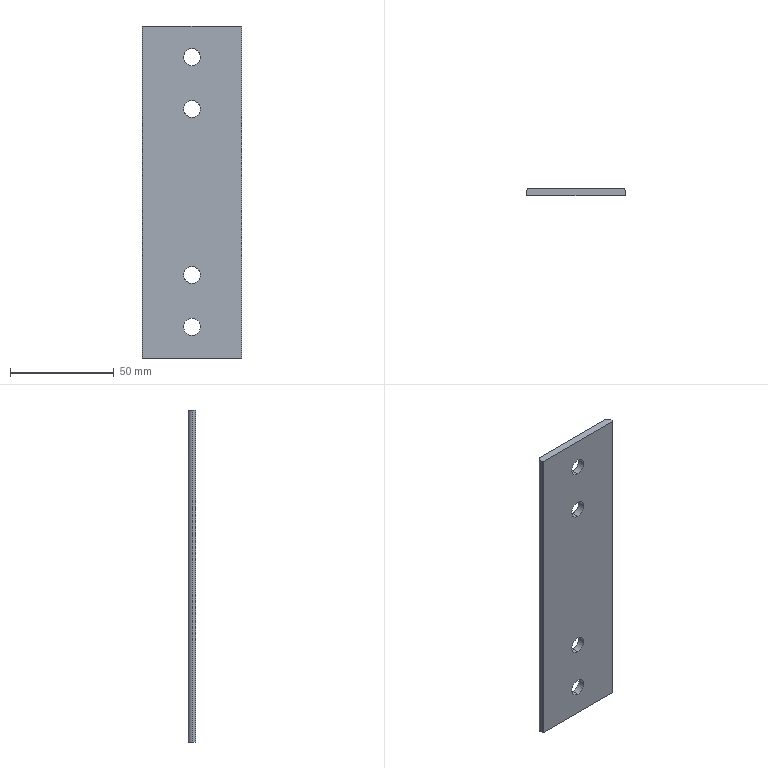Part | STEP file | 31E-01027QY13 | 1 solid | 18 faces | box 48 x 3.5 x 160 mm | volume 25860 mm3 | cylinder 12 | plane 6 | commonest cylinder face diameters 8.2 x8 0.6 x2 4 x2
STEP:
#1=CARTESIAN_POINT('',(0.,-1.75,10.9));
#2=VERTEX_POINT('',#1);
#3=CARTESIAN_POINT('',(0.,-1.75,19.1));
#4=VERTEX_POINT('',#3);
#5=CARTESIAN_POINT('',(0.,-1.75,15.));
#6=DIRECTION('',(0.,1.,0.));
#7=AXIS2_PLACEMENT_3D('',#5,#6,$);
#8=CIRCLE('',#7,4.1);
#9=EDGE_CURVE('',#2,#4,#8,.T.);
#10=ORIENTED_EDGE('',*,*,#9,.F.);
#11=CARTESIAN_POINT('',(0.,1.75,10.9));
#12=VERTEX_POINT('',#11);
#13=CARTESIAN_POINT('',(0.,-1.75,10.9));
#14=DIRECTION('',(0.,1.,0.));
#15=VECTOR('',#14,1.);
#16=LINE('',#13,#15);
#17=EDGE_CURVE('',#2,#12,#16,.T.);
#18=ORIENTED_EDGE('',*,*,#17,.T.);
#19=CARTESIAN_POINT('',(0.,1.75,19.1));
#20=VERTEX_POINT('',#19);
#21=CARTESIAN_POINT('',(0.,1.75,15.));
#22=DIRECTION('',(0.,1.,0.));
#23=AXIS2_PLACEMENT_3D('',#21,#22,$);
#24=CIRCLE('',#23,4.1);
#25=EDGE_CURVE('',#12,#20,#24,.T.);
#26=ORIENTED_EDGE('',*,*,#25,.T.);
#27=CARTESIAN_POINT('',(0.,-1.75,19.1));
#28=DIRECTION('',(0.,1.,0.));
#29=VECTOR('',#28,1.);
#30=LINE('',#27,#29);
#31=EDGE_CURVE('',#4,#20,#30,.T.);
#32=ORIENTED_EDGE('',*,*,#31,.F.);
#33=EDGE_LOOP('',(#10,#18,#26,#32));
#34=FACE_OUTER_BOUND('',#33,.T.);
#35=CARTESIAN_POINT('',(0.,-1.75,15.));
#36=DIRECTION('',(0.,1.,0.));
#37=DIRECTION('',(0.,0.,-1.));
#38=AXIS2_PLACEMENT_3D('',#35,#36,#37);
#39=CYLINDRICAL_SURFACE('',#38,4.1);
#40=ADVANCED_FACE('',(#34),#39,.F.);
#41=CARTESIAN_POINT('',(-23.7,-1.75,160.));
#42=VERTEX_POINT('',#41);
#43=CARTESIAN_POINT('',(23.7,-1.75,160.));
#44=VERTEX_POINT('',#43);
#45=CARTESIAN_POINT('',(0.,-1.75,160.));
#46=DIRECTION('',(1.,0.,0.));
#47=VECTOR('',#46,1.);
#48=LINE('',#45,#47);
#49=EDGE_CURVE('',#42,#44,#48,.T.);
#50=ORIENTED_EDGE('',*,*,#49,.F.);
#51=CARTESIAN_POINT('',(-23.7,-1.75,0.));
#52=VERTEX_POINT('',#51);
#53=CARTESIAN_POINT('',(-23.7,-1.75,80.));
#54=DIRECTION('',(0.,0.,-1.));
#55=VECTOR('',#54,1.);
#56=LINE('',#53,#55);
#57=EDGE_CURVE('',#42,#52,#56,.T.);
#58=ORIENTED_EDGE('',*,*,#57,.T.);
#59=CARTESIAN_POINT('',(23.7,-1.75,0.));
#60=VERTEX_POINT('',#59);
#61=CARTESIAN_POINT('',(0.,-1.75,0.));
#62=DIRECTION('',(1.,0.,0.));
#63=VECTOR('',#62,1.);
#64=LINE('',#61,#63);
#65=EDGE_CURVE('',#52,#60,#64,.T.);
#66=ORIENTED_EDGE('',*,*,#65,.T.);
#67=CARTESIAN_POINT('',(23.7,-1.75,80.));
#68=DIRECTION('',(0.,0.,1.));
#69=VECTOR('',#68,1.);
#70=LINE('',#67,#69);
#71=EDGE_CURVE('',#60,#44,#70,.T.);
#72=ORIENTED_EDGE('',*,*,#71,.T.);
#73=EDGE_LOOP('',(#50,#58,#66,#72));
#74=FACE_OUTER_BOUND('',#73,.T.);
#75=CARTESIAN_POINT('',(0.,-1.75,15.));
#76=DIRECTION('',(0.,1.,0.));
#77=AXIS2_PLACEMENT_3D('',#75,#76,$);
#78=CIRCLE('',#77,4.1);
#79=EDGE_CURVE('',#4,#2,#78,.T.);
#80=ORIENTED_EDGE('',*,*,#79,.T.);
#81=ORIENTED_EDGE('',*,*,#9,.T.);
#82=EDGE_LOOP('',(#80,#81));
#83=FACE_BOUND('',#82,.T.);
#84=CARTESIAN_POINT('',(0.,-1.75,44.1));
#85=VERTEX_POINT('',#84);
#86=CARTESIAN_POINT('',(0.,-1.75,35.9));
#87=VERTEX_POINT('',#86);
#88=CARTESIAN_POINT('',(0.,-1.75,40.));
#89=DIRECTION('',(0.,1.,0.));
#90=AXIS2_PLACEMENT_3D('',#88,#89,$);
#91=CIRCLE('',#90,4.1);
#92=EDGE_CURVE('',#85,#87,#91,.T.);
#93=ORIENTED_EDGE('',*,*,#92,.T.);
#94=CARTESIAN_POINT('',(0.,-1.75,40.));
#95=DIRECTION('',(0.,1.,0.));
#96=AXIS2_PLACEMENT_3D('',#94,#95,$);
#97=CIRCLE('',#96,4.1);
#98=EDGE_CURVE('',#87,#85,#97,.T.);
#99=ORIENTED_EDGE('',*,*,#98,.T.);
#100=EDGE_LOOP('',(#93,#99));
#101=FACE_BOUND('',#100,.T.);
#102=CARTESIAN_POINT('',(0.,-1.75,149.1));
#103=VERTEX_POINT('',#102);
#104=CARTESIAN_POINT('',(0.,-1.75,140.9));
#105=VERTEX_POINT('',#104);
#106=CARTESIAN_POINT('',(0.,-1.75,145.));
#107=DIRECTION('',(0.,1.,0.));
#108=AXIS2_PLACEMENT_3D('',#106,#107,$);
#109=CIRCLE('',#108,4.1);
#110=EDGE_CURVE('',#103,#105,#109,.T.);
#111=ORIENTED_EDGE('',*,*,#110,.T.);
#112=CARTESIAN_POINT('',(0.,-1.75,145.));
#113=DIRECTION('',(0.,1.,0.));
#114=AXIS2_PLACEMENT_3D('',#112,#113,$);
#115=CIRCLE('',#114,4.1);
#116=EDGE_CURVE('',#105,#103,#115,.T.);
#117=ORIENTED_EDGE('',*,*,#116,.T.);
#118=EDGE_LOOP('',(#111,#117));
#119=FACE_BOUND('',#118,.T.);
#120=CARTESIAN_POINT('',(0.,-1.75,124.1));
#121=VERTEX_POINT('',#120);
#122=CARTESIAN_POINT('',(0.,-1.75,115.9));
#123=VERTEX_POINT('',#122);
#124=CARTESIAN_POINT('',(0.,-1.75,120.));
#125=DIRECTION('',(0.,1.,0.));
#126=AXIS2_PLACEMENT_3D('',#124,#125,$);
#127=CIRCLE('',#126,4.1);
#128=EDGE_CURVE('',#121,#123,#127,.T.);
#129=ORIENTED_EDGE('',*,*,#128,.T.);
#130=CARTESIAN_POINT('',(0.,-1.75,120.));
#131=DIRECTION('',(0.,1.,0.));
#132=AXIS2_PLACEMENT_3D('',#130,#131,$);
#133=CIRCLE('',#132,4.1);
#134=EDGE_CURVE('',#123,#121,#133,.T.);
#135=ORIENTED_EDGE('',*,*,#134,.T.);
#136=EDGE_LOOP('',(#129,#135));
#137=FACE_BOUND('',#136,.T.);
#138=CARTESIAN_POINT('',(-24.,-1.75,160.));
#139=DIRECTION('',(0.,1.,0.));
#140=DIRECTION('',(0.,0.,1.));
#141=AXIS2_PLACEMENT_3D('',#138,#139,#140);
#142=PLANE('',#141);
#143=ADVANCED_FACE('',(#74,#83,#101,#119,#137),#142,.F.);
#144=ORIENTED_EDGE('',*,*,#17,.F.);
#145=ORIENTED_EDGE('',*,*,#79,.F.);
#146=ORIENTED_EDGE('',*,*,#31,.T.);
#147=CARTESIAN_POINT('',(0.,1.75,15.));
#148=DIRECTION('',(0.,1.,0.));
#149=AXIS2_PLACEMENT_3D('',#147,#148,$);
#150=CIRCLE('',#149,4.1);
#151=EDGE_CURVE('',#20,#12,#150,.T.);
#152=ORIENTED_EDGE('',*,*,#151,.T.);
#153=EDGE_LOOP('',(#144,#145,#146,#152));
#154=FACE_OUTER_BOUND('',#153,.T.);
#155=CARTESIAN_POINT('',(0.,-1.75,15.));
#156=DIRECTION('',(0.,1.,0.));
#157=DIRECTION('',(0.,0.,1.));
#158=AXIS2_PLACEMENT_3D('',#155,#156,#157);
#159=CYLINDRICAL_SURFACE('',#158,4.1);
#160=ADVANCED_FACE('',(#154),#159,.F.);
#161=CARTESIAN_POINT('',(22.,1.75,0.));
#162=VERTEX_POINT('',#161);
#163=CARTESIAN_POINT('',(-22.,1.75,0.));
#164=VERTEX_POINT('',#163);
#165=CARTESIAN_POINT('',(0.,1.75,0.));
#166=DIRECTION('',(-1.,0.,0.));
#167=VECTOR('',#166,1.);
#168=LINE('',#165,#167);
#169=EDGE_CURVE('',#162,#164,#168,.T.);
#170=ORIENTED_EDGE('',*,*,#169,.T.);
#171=CARTESIAN_POINT('',(-22.,1.75,160.));
#172=VERTEX_POINT('',#171);
#173=CARTESIAN_POINT('',(-22.,1.75,80.));
#174=DIRECTION('',(0.,0.,1.));
#175=VECTOR('',#174,1.);
#176=LINE('',#173,#175);
#177=EDGE_CURVE('',#164,#172,#176,.T.);
#178=ORIENTED_EDGE('',*,*,#177,.T.);
#179=CARTESIAN_POINT('',(22.,1.75,160.));
#180=VERTEX_POINT('',#179);
#181=CARTESIAN_POINT('',(0.,1.75,160.));
#182=DIRECTION('',(-1.,0.,0.));
#183=VECTOR('',#182,1.);
#184=LINE('',#181,#183);
#185=EDGE_CURVE('',#180,#172,#184,.T.);
#186=ORIENTED_EDGE('',*,*,#185,.F.);
#187=CARTESIAN_POINT('',(22.,1.75,80.));
#188=DIRECTION('',(0.,0.,-1.));
#189=VECTOR('',#188,1.);
#190=LINE('',#187,#189);
#191=EDGE_CURVE('',#180,#162,#190,.T.);
#192=ORIENTED_EDGE('',*,*,#191,.T.);
#193=EDGE_LOOP('',(#170,#178,#186,#192));
#194=FACE_OUTER_BOUND('',#193,.T.);
#195=ORIENTED_EDGE('',*,*,#151,.F.);
#196=ORIENTED_EDGE('',*,*,#25,.F.);
#197=EDGE_LOOP('',(#195,#196));
#198=FACE_BOUND('',#197,.T.);
#199=CARTESIAN_POINT('',(0.,1.75,44.1));
#200=VERTEX_POINT('',#199);
#201=CARTESIAN_POINT('',(0.,1.75,35.9));
#202=VERTEX_POINT('',#201);
#203=CARTESIAN_POINT('',(0.,1.75,44.1));
#204=CARTESIAN_POINT('',(0.3968,1.75,44.1));
#205=CARTESIAN_POINT('',(0.7936,1.75,44.052));
#206=CARTESIAN_POINT('',(1.183,1.75,43.956));
#207=CARTESIAN_POINT('',(1.93,1.75,43.672));
#208=CARTESIAN_POINT('',(2.588,1.75,43.218));
#209=CARTESIAN_POINT('',(2.887,1.75,42.952));
#210=CARTESIAN_POINT('',(3.416,1.75,42.352));
#211=CARTESIAN_POINT('',(3.787,1.75,41.644));
#212=CARTESIAN_POINT('',(3.929,1.75,41.27));
#213=CARTESIAN_POINT('',(4.119,1.75,40.493));
#214=CARTESIAN_POINT('',(4.118,1.75,39.694));
#215=CARTESIAN_POINT('',(4.069,1.75,39.296));
#216=CARTESIAN_POINT('',(3.875,1.75,38.52));
#217=CARTESIAN_POINT('',(3.502,1.75,37.813));
#218=CARTESIAN_POINT('',(3.274,1.75,37.484));
#219=CARTESIAN_POINT('',(2.742,1.75,36.887));
#220=CARTESIAN_POINT('',(2.083,1.75,36.435));
#221=CARTESIAN_POINT('',(1.728,1.75,36.25));
#222=CARTESIAN_POINT('',(1.169,1.75,36.04));
#223=CARTESIAN_POINT('',(0.5857,1.75,35.935));
#224=CARTESIAN_POINT('',(0.3903,1.75,35.912));
#225=CARTESIAN_POINT('',(0.1952,1.75,35.9));
#226=CARTESIAN_POINT('',(0.,1.75,35.9));
#227=B_SPLINE_CURVE_WITH_KNOTS('',5,(#203,#204,#205,#206,#207,#208,#209,#210,#211,#212,#213,#214,#215,#216,#217,#218,#219,#220,#221,#222,#223,#224,#225,#226),.UNSPECIFIED.,.F.,.U.,(6,3,3,3,3,3,3,6),(0.,2.806,5.611,8.417,11.223,14.028,16.834,18.214),.UNSPECIFIED.);
#228=EDGE_CURVE('',#200,#202,#227,.T.);
#229=ORIENTED_EDGE('',*,*,#228,.F.);
#230=CARTESIAN_POINT('',(0.,1.75,35.9));
#231=CARTESIAN_POINT('',(-0.3968,1.75,35.9));
#232=CARTESIAN_POINT('',(-0.7936,1.75,35.948));
#233=CARTESIAN_POINT('',(-1.183,1.75,36.044));
#234=CARTESIAN_POINT('',(-1.93,1.75,36.328));
#235=CARTESIAN_POINT('',(-2.588,1.75,36.782));
#236=CARTESIAN_POINT('',(-2.887,1.75,37.048));
#237=CARTESIAN_POINT('',(-3.416,1.75,37.648));
#238=CARTESIAN_POINT('',(-3.787,1.75,38.356));
#239=CARTESIAN_POINT('',(-3.929,1.75,38.73));
#240=CARTESIAN_POINT('',(-4.119,1.75,39.507));
#241=CARTESIAN_POINT('',(-4.118,1.75,40.306));
#242=CARTESIAN_POINT('',(-4.069,1.75,40.704));
#243=CARTESIAN_POINT('',(-3.875,1.75,41.48));
#244=CARTESIAN_POINT('',(-3.502,1.75,42.187));
#245=CARTESIAN_POINT('',(-3.274,1.75,42.516));
#246=CARTESIAN_POINT('',(-2.742,1.75,43.113));
#247=CARTESIAN_POINT('',(-2.083,1.75,43.565));
#248=CARTESIAN_POINT('',(-1.728,1.75,43.75));
#249=CARTESIAN_POINT('',(-1.169,1.75,43.96));
#250=CARTESIAN_POINT('',(-0.5857,1.75,44.065));
#251=CARTESIAN_POINT('',(-0.3903,1.75,44.088));
#252=CARTESIAN_POINT('',(-0.1952,1.75,44.1));
#253=CARTESIAN_POINT('',(0.,1.75,44.1));
#254=B_SPLINE_CURVE_WITH_KNOTS('',5,(#230,#231,#232,#233,#234,#235,#236,#237,#238,#239,#240,#241,#242,#243,#244,#245,#246,#247,#248,#249,#250,#251,#252,#253),.UNSPECIFIED.,.F.,.U.,(6,3,3,3,3,3,3,6),(0.,2.806,5.611,8.417,11.223,14.028,16.834,18.214),.UNSPECIFIED.);
#255=EDGE_CURVE('',#202,#200,#254,.T.);
#256=ORIENTED_EDGE('',*,*,#255,.F.);
#257=EDGE_LOOP('',(#229,#256));
#258=FACE_BOUND('',#257,.T.);
#259=CARTESIAN_POINT('',(0.,1.75,149.1));
#260=VERTEX_POINT('',#259);
#261=CARTESIAN_POINT('',(0.,1.75,140.9));
#262=VERTEX_POINT('',#261);
#263=CARTESIAN_POINT('',(0.,1.75,149.1));
#264=CARTESIAN_POINT('',(0.3968,1.75,149.1));
#265=CARTESIAN_POINT('',(0.7936,1.75,149.052));
#266=CARTESIAN_POINT('',(1.183,1.75,148.956));
#267=CARTESIAN_POINT('',(1.93,1.75,148.672));
#268=CARTESIAN_POINT('',(2.588,1.75,148.218));
#269=CARTESIAN_POINT('',(2.887,1.75,147.952));
#270=CARTESIAN_POINT('',(3.416,1.75,147.352));
#271=CARTESIAN_POINT('',(3.787,1.75,146.644));
#272=CARTESIAN_POINT('',(3.929,1.75,146.27));
#273=CARTESIAN_POINT('',(4.119,1.75,145.493));
#274=CARTESIAN_POINT('',(4.118,1.75,144.694));
#275=CARTESIAN_POINT('',(4.069,1.75,144.296));
#276=CARTESIAN_POINT('',(3.875,1.75,143.52));
#277=CARTESIAN_POINT('',(3.502,1.75,142.813));
#278=CARTESIAN_POINT('',(3.274,1.75,142.484));
#279=CARTESIAN_POINT('',(2.742,1.75,141.887));
#280=CARTESIAN_POINT('',(2.083,1.75,141.435));
#281=CARTESIAN_POINT('',(1.728,1.75,141.25));
#282=CARTESIAN_POINT('',(1.169,1.75,141.04));
#283=CARTESIAN_POINT('',(0.5857,1.75,140.935));
#284=CARTESIAN_POINT('',(0.3903,1.75,140.912));
#285=CARTESIAN_POINT('',(0.1952,1.75,140.9));
#286=CARTESIAN_POINT('',(0.,1.75,140.9));
#287=B_SPLINE_CURVE_WITH_KNOTS('',5,(#263,#264,#265,#266,#267,#268,#269,#270,#271,#272,#273,#274,#275,#276,#277,#278,#279,#280,#281,#282,#283,#284,#285,#286),.UNSPECIFIED.,.F.,.U.,(6,3,3,3,3,3,3,6),(0.,2.806,5.611,8.417,11.223,14.028,16.834,18.214),.UNSPECIFIED.);
#288=EDGE_CURVE('',#260,#262,#287,.T.);
#289=ORIENTED_EDGE('',*,*,#288,.F.);
#290=CARTESIAN_POINT('',(0.,1.75,140.9));
#291=CARTESIAN_POINT('',(-0.3968,1.75,140.9));
#292=CARTESIAN_POINT('',(-0.7936,1.75,140.948));
#293=CARTESIAN_POINT('',(-1.183,1.75,141.044));
#294=CARTESIAN_POINT('',(-1.93,1.75,141.328));
#295=CARTESIAN_POINT('',(-2.588,1.75,141.782));
#296=CARTESIAN_POINT('',(-2.887,1.75,142.048));
#297=CARTESIAN_POINT('',(-3.416,1.75,142.648));
#298=CARTESIAN_POINT('',(-3.787,1.75,143.356));
#299=CARTESIAN_POINT('',(-3.929,1.75,143.73));
#300=CARTESIAN_POINT('',(-4.119,1.75,144.507));
#301=CARTESIAN_POINT('',(-4.118,1.75,145.306));
#302=CARTESIAN_POINT('',(-4.069,1.75,145.704));
#303=CARTESIAN_POINT('',(-3.875,1.75,146.48));
#304=CARTESIAN_POINT('',(-3.502,1.75,147.187));
#305=CARTESIAN_POINT('',(-3.274,1.75,147.516));
#306=CARTESIAN_POINT('',(-2.742,1.75,148.113));
#307=CARTESIAN_POINT('',(-2.083,1.75,148.565));
#308=CARTESIAN_POINT('',(-1.728,1.75,148.75));
#309=CARTESIAN_POINT('',(-1.169,1.75,148.96));
#310=CARTESIAN_POINT('',(-0.5857,1.75,149.065));
#311=CARTESIAN_POINT('',(-0.3903,1.75,149.088));
#312=CARTESIAN_POINT('',(-0.1952,1.75,149.1));
#313=CARTESIAN_POINT('',(0.,1.75,149.1));
#314=B_SPLINE_CURVE_WITH_KNOTS('',5,(#290,#291,#292,#293,#294,#295,#296,#297,#298,#299,#300,#301,#302,#303,#304,#305,#306,#307,#308,#309,#310,#311,#312,#313),.UNSPECIFIED.,.F.,.U.,(6,3,3,3,3,3,3,6),(0.,2.806,5.611,8.417,11.223,14.028,16.834,18.214),.UNSPECIFIED.);
#315=EDGE_CURVE('',#262,#260,#314,.T.);
#316=ORIENTED_EDGE('',*,*,#315,.F.);
#317=EDGE_LOOP('',(#289,#316));
#318=FACE_BOUND('',#317,.T.);
#319=CARTESIAN_POINT('',(0.,1.75,124.1));
#320=VERTEX_POINT('',#319);
#321=CARTESIAN_POINT('',(0.,1.75,115.9));
#322=VERTEX_POINT('',#321);
#323=CARTESIAN_POINT('',(0.,1.75,124.1));
#324=CARTESIAN_POINT('',(0.3968,1.75,124.1));
#325=CARTESIAN_POINT('',(0.7936,1.75,124.052));
#326=CARTESIAN_POINT('',(1.183,1.75,123.956));
#327=CARTESIAN_POINT('',(1.93,1.75,123.672));
#328=CARTESIAN_POINT('',(2.588,1.75,123.218));
#329=CARTESIAN_POINT('',(2.887,1.75,122.952));
#330=CARTESIAN_POINT('',(3.416,1.75,122.352));
#331=CARTESIAN_POINT('',(3.787,1.75,121.644));
#332=CARTESIAN_POINT('',(3.929,1.75,121.27));
#333=CARTESIAN_POINT('',(4.119,1.75,120.493));
#334=CARTESIAN_POINT('',(4.118,1.75,119.694));
#335=CARTESIAN_POINT('',(4.069,1.75,119.296));
#336=CARTESIAN_POINT('',(3.875,1.75,118.52));
#337=CARTESIAN_POINT('',(3.502,1.75,117.813));
#338=CARTESIAN_POINT('',(3.274,1.75,117.484));
#339=CARTESIAN_POINT('',(2.742,1.75,116.887));
#340=CARTESIAN_POINT('',(2.083,1.75,116.435));
#341=CARTESIAN_POINT('',(1.728,1.75,116.25));
#342=CARTESIAN_POINT('',(1.169,1.75,116.04));
#343=CARTESIAN_POINT('',(0.5857,1.75,115.935));
#344=CARTESIAN_POINT('',(0.3903,1.75,115.912));
#345=CARTESIAN_POINT('',(0.1952,1.75,115.9));
#346=CARTESIAN_POINT('',(0.,1.75,115.9));
#347=B_SPLINE_CURVE_WITH_KNOTS('',5,(#323,#324,#325,#326,#327,#328,#329,#330,#331,#332,#333,#334,#335,#336,#337,#338,#339,#340,#341,#342,#343,#344,#345,#346),.UNSPECIFIED.,.F.,.U.,(6,3,3,3,3,3,3,6),(0.,2.806,5.611,8.417,11.223,14.028,16.834,18.214),.UNSPECIFIED.);
#348=EDGE_CURVE('',#320,#322,#347,.T.);
#349=ORIENTED_EDGE('',*,*,#348,.F.);
#350=CARTESIAN_POINT('',(0.,1.75,115.9));
#351=CARTESIAN_POINT('',(-0.3968,1.75,115.9));
#352=CARTESIAN_POINT('',(-0.7936,1.75,115.948));
#353=CARTESIAN_POINT('',(-1.183,1.75,116.044));
#354=CARTESIAN_POINT('',(-1.93,1.75,116.328));
#355=CARTESIAN_POINT('',(-2.588,1.75,116.782));
#356=CARTESIAN_POINT('',(-2.887,1.75,117.048));
#357=CARTESIAN_POINT('',(-3.416,1.75,117.648));
#358=CARTESIAN_POINT('',(-3.787,1.75,118.356));
#359=CARTESIAN_POINT('',(-3.929,1.75,118.73));
#360=CARTESIAN_POINT('',(-4.119,1.75,119.507));
#361=CARTESIAN_POINT('',(-4.118,1.75,120.306));
#362=CARTESIAN_POINT('',(-4.069,1.75,120.704));
#363=CARTESIAN_POINT('',(-3.875,1.75,121.48));
#364=CARTESIAN_POINT('',(-3.502,1.75,122.187));
#365=CARTESIAN_POINT('',(-3.274,1.75,122.516));
#366=CARTESIAN_POINT('',(-2.742,1.75,123.113));
#367=CARTESIAN_POINT('',(-2.083,1.75,123.565));
#368=CARTESIAN_POINT('',(-1.728,1.75,123.75));
#369=CARTESIAN_POINT('',(-1.169,1.75,123.96));
#370=CARTESIAN_POINT('',(-0.5857,1.75,124.065));
#371=CARTESIAN_POINT('',(-0.3903,1.75,124.088));
#372=CARTESIAN_POINT('',(-0.1952,1.75,124.1));
#373=CARTESIAN_POINT('',(0.,1.75,124.1));
#374=B_SPLINE_CURVE_WITH_KNOTS('',5,(#350,#351,#352,#353,#354,#355,#356,#357,#358,#359,#360,#361,#362,#363,#364,#365,#366,#367,#368,#369,#370,#371,#372,#373),.UNSPECIFIED.,.F.,.U.,(6,3,3,3,3,3,3,6),(0.,2.806,5.611,8.417,11.223,14.028,16.834,18.214),.UNSPECIFIED.);
#375=EDGE_CURVE('',#322,#320,#374,.T.);
#376=ORIENTED_EDGE('',*,*,#375,.F.);
#377=EDGE_LOOP('',(#349,#376));
#378=FACE_BOUND('',#377,.T.);
#379=CARTESIAN_POINT('',(-24.,1.75,160.));
#380=DIRECTION('',(0.,-1.,0.));
#381=DIRECTION('',(0.,0.,-1.));
#382=AXIS2_PLACEMENT_3D('',#379,#380,#381);
#383=PLANE('',#382);
#384=ADVANCED_FACE('',(#194,#198,#258,#318,#378),#383,.F.);
#385=CARTESIAN_POINT('',(-24.,-0.25,160.));
#386=VERTEX_POINT('',#385);
#387=CARTESIAN_POINT('',(-24.,-1.45,160.));
#388=VERTEX_POINT('',#387);
#389=CARTESIAN_POINT('',(-24.,-0.85,160.));
#390=DIRECTION('',(0.,-1.,0.));
#391=VECTOR('',#390,1.);
#392=LINE('',#389,#391);
#393=EDGE_CURVE('',#386,#388,#392,.T.);
#394=ORIENTED_EDGE('',*,*,#393,.T.);
#395=CARTESIAN_POINT('',(-23.7,-1.45,160.));
#396=DIRECTION('',(0.,0.,1.));
#397=AXIS2_PLACEMENT_3D('',#395,#396,$);
#398=CIRCLE('',#397,0.3);
#399=EDGE_CURVE('',#388,#42,#398,.T.);
#400=ORIENTED_EDGE('',*,*,#399,.T.);
#401=ORIENTED_EDGE('',*,*,#49,.T.);
#402=CARTESIAN_POINT('',(24.,-1.45,160.));
#403=VERTEX_POINT('',#402);
#404=CARTESIAN_POINT('',(23.7,-1.45,160.));
#405=DIRECTION('',(0.,0.,1.));
#406=AXIS2_PLACEMENT_3D('',#404,#405,$);
#407=CIRCLE('',#406,0.3);
#408=EDGE_CURVE('',#44,#403,#407,.T.);
#409=ORIENTED_EDGE('',*,*,#408,.T.);
#410=CARTESIAN_POINT('',(24.,-0.25,160.));
#411=VERTEX_POINT('',#410);
#412=CARTESIAN_POINT('',(24.,-0.85,160.));
#413=DIRECTION('',(0.,1.,0.));
#414=VECTOR('',#413,1.);
#415=LINE('',#412,#414);
#416=EDGE_CURVE('',#403,#411,#415,.T.);
#417=ORIENTED_EDGE('',*,*,#416,.T.);
#418=CARTESIAN_POINT('',(22.,-0.25,160.));
#419=DIRECTION('',(0.,0.,1.));
#420=AXIS2_PLACEMENT_3D('',#418,#419,$);
#421=CIRCLE('',#420,2.);
#422=EDGE_CURVE('',#411,#180,#421,.T.);
#423=ORIENTED_EDGE('',*,*,#422,.T.);
#424=ORIENTED_EDGE('',*,*,#185,.T.);
#425=CARTESIAN_POINT('',(-22.,-0.25,160.));
#426=DIRECTION('',(0.,0.,1.));
#427=AXIS2_PLACEMENT_3D('',#425,#426,$);
#428=CIRCLE('',#427,2.);
#429=EDGE_CURVE('',#172,#386,#428,.T.);
#430=ORIENTED_EDGE('',*,*,#429,.T.);
#431=EDGE_LOOP('',(#394,#400,#401,#409,#417,#423,#424,#430));
#432=FACE_OUTER_BOUND('',#431,.T.);
#433=CARTESIAN_POINT('',(24.,-1.75,160.));
#434=DIRECTION('',(0.,0.,1.));
#435=DIRECTION('',(1.,0.,0.));
#436=AXIS2_PLACEMENT_3D('',#433,#434,#435);
#437=PLANE('',#436);
#438=ADVANCED_FACE('',(#432),#437,.T.);
#439=ORIENTED_EDGE('',*,*,#399,.F.);
#440=CARTESIAN_POINT('',(-24.,-1.45,0.));
#441=VERTEX_POINT('',#440);
#442=CARTESIAN_POINT('',(-24.,-1.45,160.));
#443=DIRECTION('',(0.,0.,-1.));
#444=VECTOR('',#443,1.);
#445=LINE('',#442,#444);
#446=EDGE_CURVE('',#441,#388,#445,.F.);
#447=ORIENTED_EDGE('',*,*,#446,.F.);
#448=CARTESIAN_POINT('',(-23.7,-1.45,0.));
#449=DIRECTION('',(0.,0.,-1.));
#450=AXIS2_PLACEMENT_3D('',#448,#449,$);
#451=CIRCLE('',#450,0.3);
#452=EDGE_CURVE('',#52,#441,#451,.T.);
#453=ORIENTED_EDGE('',*,*,#452,.F.);
#454=ORIENTED_EDGE('',*,*,#57,.F.);
#455=EDGE_LOOP('',(#439,#447,#453,#454));
#456=FACE_OUTER_BOUND('',#455,.T.);
#457=CARTESIAN_POINT('',(-23.7,-1.45,160.));
#458=DIRECTION('',(0.,0.,-1.));
#459=DIRECTION('',(1.,0.,0.));
#460=AXIS2_PLACEMENT_3D('',#457,#458,#459);
#461=CYLINDRICAL_SURFACE('',#460,0.3);
#462=ADVANCED_FACE('',(#456),#461,.T.);
#463=ORIENTED_EDGE('',*,*,#65,.F.);
#464=ORIENTED_EDGE('',*,*,#452,.T.);
#465=CARTESIAN_POINT('',(-24.,-0.25,0.));
#466=VERTEX_POINT('',#465);
#467=CARTESIAN_POINT('',(-24.,-0.85,0.));
#468=DIRECTION('',(0.,-1.,0.));
#469=VECTOR('',#468,1.);
#470=LINE('',#467,#469);
#471=EDGE_CURVE('',#466,#441,#470,.T.);
#472=ORIENTED_EDGE('',*,*,#471,.F.);
#473=CARTESIAN_POINT('',(-24.,-0.25,0.));
#474=CARTESIAN_POINT('',(-24.,-0.04216,0.));
#475=CARTESIAN_POINT('',(-23.973,0.1657,0.));
#476=CARTESIAN_POINT('',(-23.919,0.3689,0.));
#477=CARTESIAN_POINT('',(-23.759,0.7565,0.));
#478=CARTESIAN_POINT('',(-23.506,1.091,0.));
#479=CARTESIAN_POINT('',(-23.358,1.24,0.));
#480=CARTESIAN_POINT('',(-23.027,1.497,0.));
#481=CARTESIAN_POINT('',(-22.642,1.661,0.));
#482=CARTESIAN_POINT('',(-22.439,1.718,0.));
#483=CARTESIAN_POINT('',(-22.227,1.748,0.));
#484=CARTESIAN_POINT('',(-22.014,1.75,0.));
#485=CARTESIAN_POINT('',(-22.01,1.75,0.));
#486=CARTESIAN_POINT('',(-22.005,1.75,0.));
#487=CARTESIAN_POINT('',(-22.,1.75,0.));
#488=B_SPLINE_CURVE_WITH_KNOTS('',5,(#473,#474,#475,#476,#477,#478,#479,#480,#481,#482,#483,#484,#485,#486,#487),.UNSPECIFIED.,.F.,.U.,(6,3,3,3,6),(0.,1.47,2.939,4.409,4.443),.UNSPECIFIED.);
#489=EDGE_CURVE('',#466,#164,#488,.T.);
#490=ORIENTED_EDGE('',*,*,#489,.T.);
#491=ORIENTED_EDGE('',*,*,#169,.F.);
#492=CARTESIAN_POINT('',(24.,-0.25,0.));
#493=VERTEX_POINT('',#492);
#494=CARTESIAN_POINT('',(22.,1.75,0.));
#495=CARTESIAN_POINT('',(22.208,1.75,0.));
#496=CARTESIAN_POINT('',(22.416,1.723,0.));
#497=CARTESIAN_POINT('',(22.619,1.669,0.));
#498=CARTESIAN_POINT('',(23.006,1.509,0.));
#499=CARTESIAN_POINT('',(23.341,1.256,0.));
#500=CARTESIAN_POINT('',(23.49,1.108,0.));
#501=CARTESIAN_POINT('',(23.747,0.7775,0.));
#502=CARTESIAN_POINT('',(23.911,0.3918,0.));
#503=CARTESIAN_POINT('',(23.968,0.1892,0.));
#504=CARTESIAN_POINT('',(23.998,-0.02304,0.));
#505=CARTESIAN_POINT('',(24.,-0.2357,0.));
#506=CARTESIAN_POINT('',(24.,-0.2404,0.));
#507=CARTESIAN_POINT('',(24.,-0.2452,0.));
#508=CARTESIAN_POINT('',(24.,-0.25,0.));
#509=B_SPLINE_CURVE_WITH_KNOTS('',5,(#494,#495,#496,#497,#498,#499,#500,#501,#502,#503,#504,#505,#506,#507,#508),.UNSPECIFIED.,.F.,.U.,(6,3,3,3,6),(0.,1.47,2.939,4.409,4.443),.UNSPECIFIED.);
#510=EDGE_CURVE('',#162,#493,#509,.T.);
#511=ORIENTED_EDGE('',*,*,#510,.T.);
#512=CARTESIAN_POINT('',(24.,-1.45,0.));
#513=VERTEX_POINT('',#512);
#514=CARTESIAN_POINT('',(24.,-0.85,0.));
#515=DIRECTION('',(0.,1.,0.));
#516=VECTOR('',#515,1.);
#517=LINE('',#514,#516);
#518=EDGE_CURVE('',#513,#493,#517,.T.);
#519=ORIENTED_EDGE('',*,*,#518,.F.);
#520=CARTESIAN_POINT('',(24.,-1.45,0.));
#521=CARTESIAN_POINT('',(24.,-1.487,0.));
#522=CARTESIAN_POINT('',(23.994,-1.525,0.));
#523=CARTESIAN_POINT('',(23.982,-1.562,0.));
#524=CARTESIAN_POINT('',(23.947,-1.63,0.));
#525=CARTESIAN_POINT('',(23.894,-1.683,0.));
#526=CARTESIAN_POINT('',(23.862,-1.707,0.));
#527=CARTESIAN_POINT('',(23.811,-1.732,0.));
#528=CARTESIAN_POINT('',(23.756,-1.746,0.));
#529=CARTESIAN_POINT('',(23.738,-1.749,0.));
#530=CARTESIAN_POINT('',(23.719,-1.75,0.));
#531=CARTESIAN_POINT('',(23.7,-1.75,0.));
#532=B_SPLINE_CURVE_WITH_KNOTS('',5,(#520,#521,#522,#523,#524,#525,#526,#527,#528,#529,#530,#531),.UNSPECIFIED.,.F.,.U.,(6,3,3,6),(0.,0.2644,0.5288,0.6618),.UNSPECIFIED.);
#533=EDGE_CURVE('',#513,#60,#532,.T.);
#534=ORIENTED_EDGE('',*,*,#533,.T.);
#535=EDGE_LOOP('',(#463,#464,#472,#490,#491,#511,#519,#534));
#536=FACE_OUTER_BOUND('',#535,.T.);
#537=CARTESIAN_POINT('',(24.,-1.75,0.));
#538=DIRECTION('',(0.,0.,1.));
#539=DIRECTION('',(1.,0.,0.));
#540=AXIS2_PLACEMENT_3D('',#537,#538,#539);
#541=PLANE('',#540);
#542=ADVANCED_FACE('',(#536),#541,.F.);
#543=ORIENTED_EDGE('',*,*,#408,.F.);
#544=ORIENTED_EDGE('',*,*,#71,.F.);
#545=ORIENTED_EDGE('',*,*,#533,.F.);
#546=CARTESIAN_POINT('',(24.,-1.45,160.));
#547=DIRECTION('',(0.,0.,-1.));
#548=VECTOR('',#547,1.);
#549=LINE('',#546,#548);
#550=EDGE_CURVE('',#403,#513,#549,.T.);
#551=ORIENTED_EDGE('',*,*,#550,.F.);
#552=EDGE_LOOP('',(#543,#544,#545,#551));
#553=FACE_OUTER_BOUND('',#552,.T.);
#554=CARTESIAN_POINT('',(23.7,-1.45,160.));
#555=DIRECTION('',(0.,0.,-1.));
#556=DIRECTION('',(1.,0.,0.));
#557=AXIS2_PLACEMENT_3D('',#554,#555,#556);
#558=CYLINDRICAL_SURFACE('',#557,0.3);
#559=ADVANCED_FACE('',(#553),#558,.T.);
#560=CARTESIAN_POINT('',(0.,-1.75,35.9));
#561=DIRECTION('',(0.,1.,0.));
#562=VECTOR('',#561,1.);
#563=LINE('',#560,#562);
#564=EDGE_CURVE('',#87,#202,#563,.T.);
#565=ORIENTED_EDGE('',*,*,#564,.F.);
#566=ORIENTED_EDGE('',*,*,#92,.F.);
#567=CARTESIAN_POINT('',(0.,-1.75,44.1));
#568=DIRECTION('',(0.,1.,0.));
#569=VECTOR('',#568,1.);
#570=LINE('',#567,#569);
#571=EDGE_CURVE('',#85,#200,#570,.T.);
#572=ORIENTED_EDGE('',*,*,#571,.T.);
#573=ORIENTED_EDGE('',*,*,#228,.T.);
#574=EDGE_LOOP('',(#565,#566,#572,#573));
#575=FACE_OUTER_BOUND('',#574,.T.);
#576=CARTESIAN_POINT('',(0.,-1.75,40.));
#577=DIRECTION('',(0.,1.,0.));
#578=DIRECTION('',(0.,0.,1.));
#579=AXIS2_PLACEMENT_3D('',#576,#577,#578);
#580=CYLINDRICAL_SURFACE('',#579,4.1);
#581=ADVANCED_FACE('',(#575),#580,.F.);
#582=ORIENTED_EDGE('',*,*,#98,.F.);
#583=ORIENTED_EDGE('',*,*,#564,.T.);
#584=ORIENTED_EDGE('',*,*,#255,.T.);
#585=ORIENTED_EDGE('',*,*,#571,.F.);
#586=EDGE_LOOP('',(#582,#583,#584,#585));
#587=FACE_OUTER_BOUND('',#586,.T.);
#588=CARTESIAN_POINT('',(0.,-1.75,40.));
#589=DIRECTION('',(0.,1.,0.));
#590=DIRECTION('',(0.,0.,-1.));
#591=AXIS2_PLACEMENT_3D('',#588,#589,#590);
#592=CYLINDRICAL_SURFACE('',#591,4.1);
#593=ADVANCED_FACE('',(#587),#592,.F.);
#594=CARTESIAN_POINT('',(0.,-1.75,140.9));
#595=DIRECTION('',(0.,1.,0.));
#596=VECTOR('',#595,1.);
#597=LINE('',#594,#596);
#598=EDGE_CURVE('',#105,#262,#597,.T.);
#599=ORIENTED_EDGE('',*,*,#598,.F.);
#600=ORIENTED_EDGE('',*,*,#110,.F.);
#601=CARTESIAN_POINT('',(0.,-1.75,149.1));
#602=DIRECTION('',(0.,1.,0.));
#603=VECTOR('',#602,1.);
#604=LINE('',#601,#603);
#605=EDGE_CURVE('',#103,#260,#604,.T.);
#606=ORIENTED_EDGE('',*,*,#605,.T.);
#607=ORIENTED_EDGE('',*,*,#288,.T.);
#608=EDGE_LOOP('',(#599,#600,#606,#607));
#609=FACE_OUTER_BOUND('',#608,.T.);
#610=CARTESIAN_POINT('',(0.,-1.75,145.));
#611=DIRECTION('',(0.,1.,0.));
#612=DIRECTION('',(0.,0.,1.));
#613=AXIS2_PLACEMENT_3D('',#610,#611,#612);
#614=CYLINDRICAL_SURFACE('',#613,4.1);
#615=ADVANCED_FACE('',(#609),#614,.F.);
#616=ORIENTED_EDGE('',*,*,#116,.F.);
#617=ORIENTED_EDGE('',*,*,#598,.T.);
#618=ORIENTED_EDGE('',*,*,#315,.T.);
#619=ORIENTED_EDGE('',*,*,#605,.F.);
#620=EDGE_LOOP('',(#616,#617,#618,#619));
#621=FACE_OUTER_BOUND('',#620,.T.);
#622=CARTESIAN_POINT('',(0.,-1.75,145.));
#623=DIRECTION('',(0.,1.,0.));
#624=DIRECTION('',(0.,0.,-1.));
#625=AXIS2_PLACEMENT_3D('',#622,#623,#624);
#626=CYLINDRICAL_SURFACE('',#625,4.1);
#627=ADVANCED_FACE('',(#621),#626,.F.);
#628=CARTESIAN_POINT('',(0.,-1.75,115.9));
#629=DIRECTION('',(0.,1.,0.));
#630=VECTOR('',#629,1.);
#631=LINE('',#628,#630);
#632=EDGE_CURVE('',#123,#322,#631,.T.);
#633=ORIENTED_EDGE('',*,*,#632,.F.);
#634=ORIENTED_EDGE('',*,*,#128,.F.);
#635=CARTESIAN_POINT('',(0.,-1.75,124.1));
#636=DIRECTION('',(0.,1.,0.));
#637=VECTOR('',#636,1.);
#638=LINE('',#635,#637);
#639=EDGE_CURVE('',#121,#320,#638,.T.);
#640=ORIENTED_EDGE('',*,*,#639,.T.);
#641=ORIENTED_EDGE('',*,*,#348,.T.);
#642=EDGE_LOOP('',(#633,#634,#640,#641));
#643=FACE_OUTER_BOUND('',#642,.T.);
#644=CARTESIAN_POINT('',(0.,-1.75,120.));
#645=DIRECTION('',(0.,1.,0.));
#646=DIRECTION('',(0.,0.,1.));
#647=AXIS2_PLACEMENT_3D('',#644,#645,#646);
#648=CYLINDRICAL_SURFACE('',#647,4.1);
#649=ADVANCED_FACE('',(#643),#648,.F.);
#650=ORIENTED_EDGE('',*,*,#134,.F.);
#651=ORIENTED_EDGE('',*,*,#632,.T.);
#652=ORIENTED_EDGE('',*,*,#375,.T.);
#653=ORIENTED_EDGE('',*,*,#639,.F.);
#654=EDGE_LOOP('',(#650,#651,#652,#653));
#655=FACE_OUTER_BOUND('',#654,.T.);
#656=CARTESIAN_POINT('',(0.,-1.75,120.));
#657=DIRECTION('',(0.,1.,0.));
#658=DIRECTION('',(0.,0.,-1.));
#659=AXIS2_PLACEMENT_3D('',#656,#657,#658);
#660=CYLINDRICAL_SURFACE('',#659,4.1);
#661=ADVANCED_FACE('',(#655),#660,.F.);
#662=ORIENTED_EDGE('',*,*,#429,.F.);
#663=ORIENTED_EDGE('',*,*,#177,.F.);
#664=ORIENTED_EDGE('',*,*,#489,.F.);
#665=CARTESIAN_POINT('',(-24.,-0.25,160.));
#666=DIRECTION('',(0.,0.,-1.));
#667=VECTOR('',#666,1.);
#668=LINE('',#665,#667);
#669=EDGE_CURVE('',#386,#466,#668,.T.);
#670=ORIENTED_EDGE('',*,*,#669,.F.);
#671=EDGE_LOOP('',(#662,#663,#664,#670));
#672=FACE_OUTER_BOUND('',#671,.T.);
#673=CARTESIAN_POINT('',(-22.,-0.25,160.));
#674=DIRECTION('',(0.,0.,-1.));
#675=DIRECTION('',(-1.,0.,0.));
#676=AXIS2_PLACEMENT_3D('',#673,#674,#675);
#677=CYLINDRICAL_SURFACE('',#676,2.);
#678=ADVANCED_FACE('',(#672),#677,.T.);
#679=ORIENTED_EDGE('',*,*,#422,.F.);
#680=CARTESIAN_POINT('',(24.,-0.25,160.));
#681=DIRECTION('',(0.,0.,-1.));
#682=VECTOR('',#681,1.);
#683=LINE('',#680,#682);
#684=EDGE_CURVE('',#493,#411,#683,.F.);
#685=ORIENTED_EDGE('',*,*,#684,.F.);
#686=ORIENTED_EDGE('',*,*,#510,.F.);
#687=ORIENTED_EDGE('',*,*,#191,.F.);
#688=EDGE_LOOP('',(#679,#685,#686,#687));
#689=FACE_OUTER_BOUND('',#688,.T.);
#690=CARTESIAN_POINT('',(22.,-0.25,160.));
#691=DIRECTION('',(0.,0.,-1.));
#692=DIRECTION('',(-1.,0.,0.));
#693=AXIS2_PLACEMENT_3D('',#690,#691,#692);
#694=CYLINDRICAL_SURFACE('',#693,2.);
#695=ADVANCED_FACE('',(#689),#694,.T.);
#696=ORIENTED_EDGE('',*,*,#471,.T.);
#697=ORIENTED_EDGE('',*,*,#446,.T.);
#698=ORIENTED_EDGE('',*,*,#393,.F.);
#699=ORIENTED_EDGE('',*,*,#669,.T.);
#700=EDGE_LOOP('',(#696,#697,#698,#699));
#701=FACE_OUTER_BOUND('',#700,.T.);
#702=CARTESIAN_POINT('',(-24.,1.75,160.));
#703=DIRECTION('',(1.,0.,0.));
#704=DIRECTION('',(0.,0.,-1.));
#705=AXIS2_PLACEMENT_3D('',#702,#703,#704);
#706=PLANE('',#705);
#707=ADVANCED_FACE('',(#701),#706,.F.);
#708=ORIENTED_EDGE('',*,*,#416,.F.);
#709=ORIENTED_EDGE('',*,*,#550,.T.);
#710=ORIENTED_EDGE('',*,*,#518,.T.);
#711=ORIENTED_EDGE('',*,*,#684,.T.);
#712=EDGE_LOOP('',(#708,#709,#710,#711));
#713=FACE_OUTER_BOUND('',#712,.T.);
#714=CARTESIAN_POINT('',(24.,1.75,160.));
#715=DIRECTION('',(-1.,0.,0.));
#716=DIRECTION('',(0.,-1.,0.));
#717=AXIS2_PLACEMENT_3D('',#714,#715,#716);
#718=PLANE('',#717);
#719=ADVANCED_FACE('',(#713),#718,.F.);
#720=CLOSED_SHELL('',(#40,#143,#160,#384,#438,#462,#542,#559,#581,#593,#615,#627,#649,#661,#678,#695,#707,#719));
#721=MANIFOLD_SOLID_BREP('',#720);
#722=(LENGTH_UNIT()NAMED_UNIT(*)SI_UNIT(.MILLI.,.METRE.));
#723=UNCERTAINTY_MEASURE_WITH_UNIT(LENGTH_MEASURE(0.005),#722,'','');
#724=(NAMED_UNIT(*)PLANE_ANGLE_UNIT()SI_UNIT($,.RADIAN.));
#725=(NAMED_UNIT(*)SI_UNIT($,.STERADIAN.)SOLID_ANGLE_UNIT());
#726=(GEOMETRIC_REPRESENTATION_CONTEXT(3)GLOBAL_UNCERTAINTY_ASSIGNED_CONTEXT((#723))GLOBAL_UNIT_ASSIGNED_CONTEXT((#722,#724,#725))REPRESENTATION_CONTEXT('',''));
#727=ADVANCED_BREP_SHAPE_REPRESENTATION('',(#721),#726);